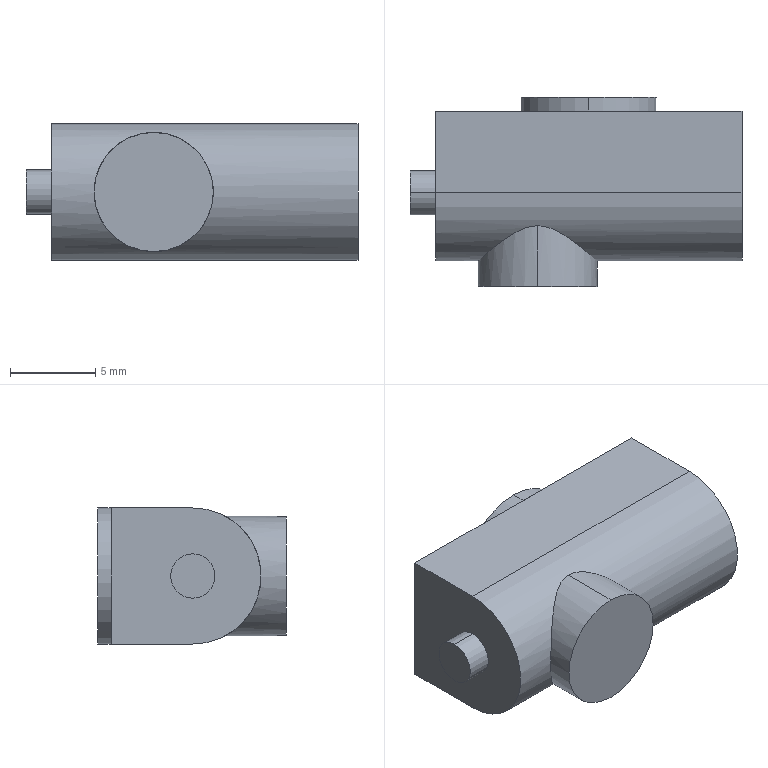Part | STEP file | AFM30-03_AFM3022A Drain_30 | 1 solid | 16 faces | box 19.5 x 11.1 x 8 mm | volume 1266 mm3 | plane 9 | cylinder 7 | commonest cylinder face diameters 8 x3 2.6 x2 7 x2
STEP:
#1=CARTESIAN_POINT('',(-10.5,-5.6,1.3));
#2=VERTEX_POINT('',#1);
#3=CARTESIAN_POINT('',(-10.5,-5.6,-1.3));
#4=VERTEX_POINT('',#3);
#5=CARTESIAN_POINT('',(-10.5,-5.6,0.));
#6=DIRECTION('',(-1.,0.,0.));
#7=DIRECTION('',(0.,0.,1.));
#8=AXIS2_PLACEMENT_3D('',#5,#6,#7);
#9=CIRCLE('',#8,1.3);
#10=EDGE_CURVE('',#2,#4,#9,.T.);
#11=ORIENTED_EDGE('',*,*,#10,.F.);
#12=CARTESIAN_POINT('',(-9.,-5.6,1.3));
#13=VERTEX_POINT('',#12);
#14=CARTESIAN_POINT('',(-10.5,-5.6,1.3));
#15=DIRECTION('',(1.,0.,0.));
#16=VECTOR('',#15,1000.);
#17=LINE('',#14,#16);
#18=EDGE_CURVE('',#2,#13,#17,.T.);
#19=ORIENTED_EDGE('',*,*,#18,.T.);
#20=CARTESIAN_POINT('',(-9.,-5.6,-1.3));
#21=VERTEX_POINT('',#20);
#22=CARTESIAN_POINT('',(-9.,-5.6,0.));
#23=DIRECTION('',(-1.,0.,0.));
#24=DIRECTION('',(0.,0.,-1.));
#25=AXIS2_PLACEMENT_3D('',#22,#23,#24);
#26=CIRCLE('',#25,1.3);
#27=EDGE_CURVE('',#13,#21,#26,.T.);
#28=ORIENTED_EDGE('',*,*,#27,.T.);
#29=CARTESIAN_POINT('',(-10.5,-5.6,-1.3));
#30=DIRECTION('',(1.,0.,0.));
#31=VECTOR('',#30,1000.);
#32=LINE('',#29,#31);
#33=EDGE_CURVE('',#4,#21,#32,.T.);
#34=ORIENTED_EDGE('',*,*,#33,.F.);
#35=EDGE_LOOP('',(#11,#19,#28,#34));
#36=FACE_OUTER_BOUND('',#35,.T.);
#37=CARTESIAN_POINT('',(-10.5,-5.6,0.));
#38=DIRECTION('',(1.,0.,0.));
#39=DIRECTION('',(0.,0.,-1.));
#40=AXIS2_PLACEMENT_3D('',#37,#38,#39);
#41=CYLINDRICAL_SURFACE('',#40,1.3);
#42=ADVANCED_FACE('',(#36),#41,.T.);
#43=CARTESIAN_POINT('',(-3.,-11.1,3.5));
#44=VERTEX_POINT('',#43);
#45=CARTESIAN_POINT('',(-3.,-11.1,-3.5));
#46=VERTEX_POINT('',#45);
#47=CARTESIAN_POINT('',(-3.,-11.1,0.));
#48=DIRECTION('',(0.,1.,0.));
#49=DIRECTION('',(0.,0.,1.));
#50=AXIS2_PLACEMENT_3D('',#47,#48,#49);
#51=CIRCLE('',#50,3.5);
#52=EDGE_CURVE('',#44,#46,#51,.T.);
#53=ORIENTED_EDGE('',*,*,#52,.T.);
#54=CARTESIAN_POINT('',(-3.,-7.536,-3.5));
#55=VERTEX_POINT('',#54);
#56=CARTESIAN_POINT('',(-3.,-11.1,-3.5));
#57=DIRECTION('',(0.,1.,0.));
#58=VECTOR('',#57,1000.);
#59=LINE('',#56,#58);
#60=EDGE_CURVE('',#46,#55,#59,.T.);
#61=ORIENTED_EDGE('',*,*,#60,.T.);
#62=CARTESIAN_POINT('',(-3.,-7.536,3.5));
#63=VERTEX_POINT('',#62);
#64=CARTESIAN_POINT('',(-3.,-7.536,3.5));
#65=CARTESIAN_POINT('',(-2.748,-7.536,3.5));
#66=CARTESIAN_POINT('',(-2.506,-7.587,3.473));
#67=CARTESIAN_POINT('',(-2.044,-7.749,3.375));
#68=CARTESIAN_POINT('',(-1.832,-7.856,3.307));
#69=CARTESIAN_POINT('',(-1.429,-8.088,3.135));
#70=CARTESIAN_POINT('',(-1.239,-8.214,3.032));
#71=CARTESIAN_POINT('',(-0.8859,-8.464,2.797));
#72=CARTESIAN_POINT('',(-0.7207,-8.589,2.665));
#73=CARTESIAN_POINT('',(-0.4108,-8.832,2.365));
#74=CARTESIAN_POINT('',(-0.2662,-8.949,2.197));
#75=CARTESIAN_POINT('',(-0.009917,-9.162,1.833));
#76=CARTESIAN_POINT('',(0.1038,-9.258,1.635));
#77=CARTESIAN_POINT('',(0.295,-9.422,1.203));
#78=CARTESIAN_POINT('',(0.3697,-9.486,0.9771));
#79=CARTESIAN_POINT('',(0.4469,-9.554,0.6193));
#80=CARTESIAN_POINT('',(0.4669,-9.571,0.4961));
#81=CARTESIAN_POINT('',(0.4932,-9.594,0.2506));
#82=CARTESIAN_POINT('',(0.4998,-9.6,0.1277));
#83=CARTESIAN_POINT('',(0.5003,-9.6,-0.2418));
#84=CARTESIAN_POINT('',(0.4737,-9.577,-0.4926));
#85=CARTESIAN_POINT('',(0.372,-9.488,-0.9689));
#86=CARTESIAN_POINT('',(0.2966,-9.423,-1.199));
#87=CARTESIAN_POINT('',(0.01172,-9.179,-1.844));
#88=CARTESIAN_POINT('',(-0.2543,-8.954,-2.213));
#89=CARTESIAN_POINT('',(-0.7164,-8.593,-2.661));
#90=CARTESIAN_POINT('',(-0.882,-8.467,-2.795));
#91=CARTESIAN_POINT('',(-1.24,-8.214,-3.033));
#92=CARTESIAN_POINT('',(-1.428,-8.089,-3.134));
#93=CARTESIAN_POINT('',(-1.829,-7.857,-3.305));
#94=CARTESIAN_POINT('',(-2.045,-7.749,-3.375));
#95=CARTESIAN_POINT('',(-2.39,-7.628,-3.448));
#96=CARTESIAN_POINT('',(-2.508,-7.594,-3.467));
#97=CARTESIAN_POINT('',(-2.752,-7.549,-3.493));
#98=CARTESIAN_POINT('',(-2.877,-7.536,-3.5));
#99=CARTESIAN_POINT('',(-3.,-7.536,-3.5));
#100=B_SPLINE_CURVE_WITH_KNOTS('',3,(#64,#65,#66,#67,#68,#69,#70,#71,#72,#73,#74,#75,#76,#77,#78,#79,#80,#81,#82,#83,#84,#85,#86,#87,#88,#89,#90,#91,#92,#93,#94,#95,#96,#97,#98,#99),.UNSPECIFIED.,.F.,.F.,(4,2,2,2,2,2,2,2,2,2,2,2,2,2,2,2,2,4),(0.,0.0007411,0.001482,0.002223,0.002964,0.003705,0.004446,0.005188,0.005558,0.005929,0.00667,0.007411,0.008893,0.009634,0.01038,0.01112,0.01149,0.01186),.UNSPECIFIED.);
#101=EDGE_CURVE('',#63,#55,#100,.T.);
#102=ORIENTED_EDGE('',*,*,#101,.F.);
#103=CARTESIAN_POINT('',(-3.,-11.1,3.5));
#104=DIRECTION('',(0.,1.,0.));
#105=VECTOR('',#104,1000.);
#106=LINE('',#103,#105);
#107=EDGE_CURVE('',#44,#63,#106,.T.);
#108=ORIENTED_EDGE('',*,*,#107,.F.);
#109=EDGE_LOOP('',(#53,#61,#102,#108));
#110=FACE_OUTER_BOUND('',#109,.T.);
#111=CARTESIAN_POINT('',(-3.,-11.1,0.));
#112=DIRECTION('',(0.,1.,0.));
#113=DIRECTION('',(0.,0.,1.));
#114=AXIS2_PLACEMENT_3D('',#111,#112,#113);
#115=CYLINDRICAL_SURFACE('',#114,3.5);
#116=ADVANCED_FACE('',(#110),#115,.T.);
#117=CARTESIAN_POINT('',(0.,-0.8,4.));
#118=VERTEX_POINT('',#117);
#119=CARTESIAN_POINT('',(0.,-0.8,-4.));
#120=VERTEX_POINT('',#119);
#121=CARTESIAN_POINT('',(0.,-0.8,0.));
#122=DIRECTION('',(0.,1.,0.));
#123=DIRECTION('',(0.,0.,1.));
#124=AXIS2_PLACEMENT_3D('',#121,#122,#123);
#125=CIRCLE('',#124,4.);
#126=EDGE_CURVE('',#118,#120,#125,.T.);
#127=ORIENTED_EDGE('',*,*,#126,.T.);
#128=CARTESIAN_POINT('',(0.,0.,-4.));
#129=VERTEX_POINT('',#128);
#130=CARTESIAN_POINT('',(0.,-0.8,-4.));
#131=DIRECTION('',(0.,1.,0.));
#132=VECTOR('',#131,1000.);
#133=LINE('',#130,#132);
#134=EDGE_CURVE('',#120,#129,#133,.T.);
#135=ORIENTED_EDGE('',*,*,#134,.T.);
#136=CARTESIAN_POINT('',(0.,0.,4.));
#137=VERTEX_POINT('',#136);
#138=CARTESIAN_POINT('',(0.,0.,0.));
#139=DIRECTION('',(0.,1.,0.));
#140=DIRECTION('',(0.,0.,1.));
#141=AXIS2_PLACEMENT_3D('',#138,#139,#140);
#142=CIRCLE('',#141,4.);
#143=EDGE_CURVE('',#137,#129,#142,.T.);
#144=ORIENTED_EDGE('',*,*,#143,.F.);
#145=CARTESIAN_POINT('',(0.,-0.8,4.));
#146=DIRECTION('',(0.,1.,0.));
#147=VECTOR('',#146,1000.);
#148=LINE('',#145,#147);
#149=EDGE_CURVE('',#118,#137,#148,.T.);
#150=ORIENTED_EDGE('',*,*,#149,.F.);
#151=EDGE_LOOP('',(#127,#135,#144,#150));
#152=FACE_OUTER_BOUND('',#151,.T.);
#153=CARTESIAN_POINT('',(0.,-0.8,0.));
#154=DIRECTION('',(0.,1.,0.));
#155=DIRECTION('',(0.,0.,1.));
#156=AXIS2_PLACEMENT_3D('',#153,#154,#155);
#157=CYLINDRICAL_SURFACE('',#156,4.);
#158=ADVANCED_FACE('',(#152),#157,.T.);
#159=CARTESIAN_POINT('',(-9.,-0.8,-4.));
#160=VERTEX_POINT('',#159);
#161=CARTESIAN_POINT('',(-9.,-0.8,4.));
#162=VERTEX_POINT('',#161);
#163=CARTESIAN_POINT('',(-9.,-0.8,4.));
#164=DIRECTION('',(0.,0.,1.));
#165=VECTOR('',#164,1000.);
#166=LINE('',#163,#165);
#167=EDGE_CURVE('',#160,#162,#166,.T.);
#168=ORIENTED_EDGE('',*,*,#167,.F.);
#169=CARTESIAN_POINT('',(-9.,-5.6,-4.));
#170=VERTEX_POINT('',#169);
#171=CARTESIAN_POINT('',(-9.,-0.8,-4.));
#172=DIRECTION('',(0.,1.,0.));
#173=VECTOR('',#172,1000.);
#174=LINE('',#171,#173);
#175=EDGE_CURVE('',#170,#160,#174,.T.);
#176=ORIENTED_EDGE('',*,*,#175,.F.);
#177=CARTESIAN_POINT('',(-9.,-5.6,4.));
#178=VERTEX_POINT('',#177);
#179=CARTESIAN_POINT('',(-9.,-5.6,0.));
#180=DIRECTION('',(1.,0.,0.));
#181=DIRECTION('',(0.,0.,-1.));
#182=AXIS2_PLACEMENT_3D('',#179,#180,#181);
#183=CIRCLE('',#182,4.);
#184=EDGE_CURVE('',#178,#170,#183,.T.);
#185=ORIENTED_EDGE('',*,*,#184,.F.);
#186=CARTESIAN_POINT('',(-9.,-0.8,4.));
#187=DIRECTION('',(0.,-1.,0.));
#188=VECTOR('',#187,1000.);
#189=LINE('',#186,#188);
#190=EDGE_CURVE('',#162,#178,#189,.T.);
#191=ORIENTED_EDGE('',*,*,#190,.F.);
#192=EDGE_LOOP('',(#168,#176,#185,#191));
#193=FACE_OUTER_BOUND('',#192,.T.);
#194=CARTESIAN_POINT('',(-9.,-5.6,0.));
#195=DIRECTION('',(-1.,0.,0.));
#196=DIRECTION('',(0.,0.,-1.));
#197=AXIS2_PLACEMENT_3D('',#194,#195,#196);
#198=CIRCLE('',#197,1.3);
#199=EDGE_CURVE('',#21,#13,#198,.T.);
#200=ORIENTED_EDGE('',*,*,#199,.F.);
#201=ORIENTED_EDGE('',*,*,#27,.F.);
#202=EDGE_LOOP('',(#200,#201));
#203=FACE_BOUND('',#202,.T.);
#204=CARTESIAN_POINT('',(-9.,-5.6,0.));
#205=DIRECTION('',(1.,0.,0.));
#206=DIRECTION('',(0.,0.,-1.));
#207=AXIS2_PLACEMENT_3D('',#204,#205,#206);
#208=PLANE('',#207);
#209=ADVANCED_FACE('',(#193,#203),#208,.F.);
#210=ORIENTED_EDGE('',*,*,#134,.F.);
#211=CARTESIAN_POINT('',(0.,-0.8,0.));
#212=DIRECTION('',(0.,1.,0.));
#213=DIRECTION('',(0.,0.,1.));
#214=AXIS2_PLACEMENT_3D('',#211,#212,#213);
#215=CIRCLE('',#214,4.);
#216=EDGE_CURVE('',#120,#118,#215,.T.);
#217=ORIENTED_EDGE('',*,*,#216,.T.);
#218=ORIENTED_EDGE('',*,*,#149,.T.);
#219=CARTESIAN_POINT('',(0.,0.,0.));
#220=DIRECTION('',(0.,1.,0.));
#221=DIRECTION('',(0.,0.,1.));
#222=AXIS2_PLACEMENT_3D('',#219,#220,#221);
#223=CIRCLE('',#222,4.);
#224=EDGE_CURVE('',#129,#137,#223,.T.);
#225=ORIENTED_EDGE('',*,*,#224,.F.);
#226=EDGE_LOOP('',(#210,#217,#218,#225));
#227=FACE_OUTER_BOUND('',#226,.T.);
#228=CARTESIAN_POINT('',(0.,-0.8,0.));
#229=DIRECTION('',(0.,1.,0.));
#230=DIRECTION('',(0.,0.,1.));
#231=AXIS2_PLACEMENT_3D('',#228,#229,#230);
#232=CYLINDRICAL_SURFACE('',#231,4.);
#233=ADVANCED_FACE('',(#227),#232,.T.);
#234=ORIENTED_EDGE('',*,*,#143,.T.);
#235=ORIENTED_EDGE('',*,*,#224,.T.);
#236=EDGE_LOOP('',(#234,#235));
#237=FACE_OUTER_BOUND('',#236,.T.);
#238=CARTESIAN_POINT('',(0.,0.,0.));
#239=DIRECTION('',(0.,1.,0.));
#240=DIRECTION('',(0.,0.,1.));
#241=AXIS2_PLACEMENT_3D('',#238,#239,#240);
#242=PLANE('',#241);
#243=ADVANCED_FACE('',(#237),#242,.T.);
#244=ORIENTED_EDGE('',*,*,#126,.F.);
#245=CARTESIAN_POINT('',(9.,-0.8,4.));
#246=VERTEX_POINT('',#245);
#247=CARTESIAN_POINT('',(9.,-0.8,4.));
#248=DIRECTION('',(-1.,0.,0.));
#249=VECTOR('',#248,1000.);
#250=LINE('',#247,#249);
#251=EDGE_CURVE('',#246,#118,#250,.T.);
#252=ORIENTED_EDGE('',*,*,#251,.F.);
#253=CARTESIAN_POINT('',(9.,-0.8,-4.));
#254=VERTEX_POINT('',#253);
#255=CARTESIAN_POINT('',(9.,-0.8,4.));
#256=DIRECTION('',(0.,0.,1.));
#257=VECTOR('',#256,1000.);
#258=LINE('',#255,#257);
#259=EDGE_CURVE('',#254,#246,#258,.T.);
#260=ORIENTED_EDGE('',*,*,#259,.F.);
#261=CARTESIAN_POINT('',(9.,-0.8,-4.));
#262=DIRECTION('',(-1.,0.,0.));
#263=VECTOR('',#262,1000.);
#264=LINE('',#261,#263);
#265=EDGE_CURVE('',#254,#120,#264,.T.);
#266=ORIENTED_EDGE('',*,*,#265,.T.);
#267=EDGE_LOOP('',(#244,#252,#260,#266));
#268=FACE_OUTER_BOUND('',#267,.T.);
#269=CARTESIAN_POINT('',(9.,-0.8,4.));
#270=DIRECTION('',(0.,-1.,0.));
#271=DIRECTION('',(0.,0.,-1.));
#272=AXIS2_PLACEMENT_3D('',#269,#270,#271);
#273=PLANE('',#272);
#274=ADVANCED_FACE('',(#268),#273,.F.);
#275=CARTESIAN_POINT('',(9.,-0.8,4.));
#276=DIRECTION('',(-1.,0.,0.));
#277=VECTOR('',#276,1000.);
#278=LINE('',#275,#277);
#279=EDGE_CURVE('',#118,#162,#278,.T.);
#280=ORIENTED_EDGE('',*,*,#279,.F.);
#281=ORIENTED_EDGE('',*,*,#216,.F.);
#282=CARTESIAN_POINT('',(9.,-0.8,-4.));
#283=DIRECTION('',(-1.,0.,0.));
#284=VECTOR('',#283,1000.);
#285=LINE('',#282,#284);
#286=EDGE_CURVE('',#120,#160,#285,.T.);
#287=ORIENTED_EDGE('',*,*,#286,.T.);
#288=ORIENTED_EDGE('',*,*,#167,.T.);
#289=EDGE_LOOP('',(#280,#281,#287,#288));
#290=FACE_OUTER_BOUND('',#289,.T.);
#291=CARTESIAN_POINT('',(9.,-0.8,4.));
#292=DIRECTION('',(0.,-1.,0.));
#293=DIRECTION('',(0.,0.,-1.));
#294=AXIS2_PLACEMENT_3D('',#291,#292,#293);
#295=PLANE('',#294);
#296=ADVANCED_FACE('',(#290),#295,.F.);
#297=ORIENTED_EDGE('',*,*,#190,.T.);
#298=CARTESIAN_POINT('',(9.,-5.6,4.));
#299=VERTEX_POINT('',#298);
#300=CARTESIAN_POINT('',(9.,-5.6,4.));
#301=DIRECTION('',(-1.,0.,0.));
#302=VECTOR('',#301,1000.);
#303=LINE('',#300,#302);
#304=EDGE_CURVE('',#299,#178,#303,.T.);
#305=ORIENTED_EDGE('',*,*,#304,.F.);
#306=CARTESIAN_POINT('',(9.,-0.8,4.));
#307=DIRECTION('',(0.,-1.,0.));
#308=VECTOR('',#307,1000.);
#309=LINE('',#306,#308);
#310=EDGE_CURVE('',#246,#299,#309,.T.);
#311=ORIENTED_EDGE('',*,*,#310,.F.);
#312=ORIENTED_EDGE('',*,*,#251,.T.);
#313=ORIENTED_EDGE('',*,*,#279,.T.);
#314=EDGE_LOOP('',(#297,#305,#311,#312,#313));
#315=FACE_OUTER_BOUND('',#314,.T.);
#316=CARTESIAN_POINT('',(9.,-0.8,4.));
#317=DIRECTION('',(0.,0.,-1.));
#318=DIRECTION('',(0.,1.,0.));
#319=AXIS2_PLACEMENT_3D('',#316,#317,#318);
#320=PLANE('',#319);
#321=ADVANCED_FACE('',(#315),#320,.F.);
#322=ORIENTED_EDGE('',*,*,#101,.T.);
#323=CARTESIAN_POINT('',(-3.,-7.536,-3.5));
#324=CARTESIAN_POINT('',(-3.247,-7.536,-3.5));
#325=CARTESIAN_POINT('',(-3.495,-7.587,-3.473));
#326=CARTESIAN_POINT('',(-3.953,-7.748,-3.376));
#327=CARTESIAN_POINT('',(-4.17,-7.857,-3.306));
#328=CARTESIAN_POINT('',(-4.571,-8.089,-3.135));
#329=CARTESIAN_POINT('',(-4.759,-8.213,-3.034));
#330=CARTESIAN_POINT('',(-5.115,-8.464,-2.797));
#331=CARTESIAN_POINT('',(-5.282,-8.592,-2.662));
#332=CARTESIAN_POINT('',(-5.59,-8.833,-2.363));
#333=CARTESIAN_POINT('',(-5.732,-8.948,-2.199));
#334=CARTESIAN_POINT('',(-5.99,-9.162,-1.832));
#335=CARTESIAN_POINT('',(-6.105,-9.259,-1.632));
#336=CARTESIAN_POINT('',(-6.294,-9.421,-1.206));
#337=CARTESIAN_POINT('',(-6.37,-9.487,-0.9741));
#338=CARTESIAN_POINT('',(-6.473,-9.576,-0.4995));
#339=CARTESIAN_POINT('',(-6.5,-9.6,-0.2562));
#340=CARTESIAN_POINT('',(-6.5,-9.6,0.2437));
#341=CARTESIAN_POINT('',(-6.474,-9.577,0.4897));
#342=CARTESIAN_POINT('',(-6.373,-9.489,0.967));
#343=CARTESIAN_POINT('',(-6.297,-9.423,1.198));
#344=CARTESIAN_POINT('',(-6.108,-9.261,1.627));
#345=CARTESIAN_POINT('',(-5.993,-9.164,1.829));
#346=CARTESIAN_POINT('',(-5.736,-8.951,2.194));
#347=CARTESIAN_POINT('',(-5.594,-8.836,2.359));
#348=CARTESIAN_POINT('',(-5.285,-8.593,2.66));
#349=CARTESIAN_POINT('',(-5.117,-8.466,2.796));
#350=CARTESIAN_POINT('',(-4.762,-8.215,3.031));
#351=CARTESIAN_POINT('',(-4.575,-8.091,3.133));
#352=CARTESIAN_POINT('',(-4.171,-7.857,3.306));
#353=CARTESIAN_POINT('',(-3.956,-7.749,3.375));
#354=CARTESIAN_POINT('',(-3.611,-7.628,3.448));
#355=CARTESIAN_POINT('',(-3.491,-7.594,3.468));
#356=CARTESIAN_POINT('',(-3.249,-7.549,3.493));
#357=CARTESIAN_POINT('',(-3.126,-7.536,3.5));
#358=CARTESIAN_POINT('',(-3.,-7.536,3.5));
#359=B_SPLINE_CURVE_WITH_KNOTS('',3,(#323,#324,#325,#326,#327,#328,#329,#330,#331,#332,#333,#334,#335,#336,#337,#338,#339,#340,#341,#342,#343,#344,#345,#346,#347,#348,#349,#350,#351,#352,#353,#354,#355,#356,#357,#358),.UNSPECIFIED.,.F.,.F.,(4,2,2,2,2,2,2,2,2,2,2,2,2,2,2,2,2,4),(0.01186,0.0126,0.01334,0.01408,0.01482,0.01556,0.0163,0.01704,0.01778,0.01853,0.01927,0.02001,0.02075,0.02149,0.02223,0.02297,0.02334,0.02371),.UNSPECIFIED.);
#360=EDGE_CURVE('',#55,#63,#359,.T.);
#361=ORIENTED_EDGE('',*,*,#360,.T.);
#362=EDGE_LOOP('',(#322,#361));
#363=FACE_BOUND('',#362,.T.);
#364=ORIENTED_EDGE('',*,*,#184,.T.);
#365=CARTESIAN_POINT('',(9.,-5.6,-4.));
#366=VERTEX_POINT('',#365);
#367=CARTESIAN_POINT('',(9.,-5.6,-4.));
#368=DIRECTION('',(-1.,0.,0.));
#369=VECTOR('',#368,1000.);
#370=LINE('',#367,#369);
#371=EDGE_CURVE('',#366,#170,#370,.T.);
#372=ORIENTED_EDGE('',*,*,#371,.F.);
#373=CARTESIAN_POINT('',(9.,-5.6,0.));
#374=DIRECTION('',(1.,0.,0.));
#375=DIRECTION('',(0.,0.,-1.));
#376=AXIS2_PLACEMENT_3D('',#373,#374,#375);
#377=CIRCLE('',#376,4.);
#378=EDGE_CURVE('',#299,#366,#377,.T.);
#379=ORIENTED_EDGE('',*,*,#378,.F.);
#380=ORIENTED_EDGE('',*,*,#304,.T.);
#381=EDGE_LOOP('',(#364,#372,#379,#380));
#382=FACE_OUTER_BOUND('',#381,.T.);
#383=CARTESIAN_POINT('',(9.,-5.6,0.));
#384=DIRECTION('',(-1.,0.,0.));
#385=DIRECTION('',(0.,0.,1.));
#386=AXIS2_PLACEMENT_3D('',#383,#384,#385);
#387=CYLINDRICAL_SURFACE('',#386,4.);
#388=ADVANCED_FACE('',(#363,#382),#387,.T.);
#389=ORIENTED_EDGE('',*,*,#175,.T.);
#390=ORIENTED_EDGE('',*,*,#286,.F.);
#391=ORIENTED_EDGE('',*,*,#265,.F.);
#392=CARTESIAN_POINT('',(9.,-0.8,-4.));
#393=DIRECTION('',(0.,1.,0.));
#394=VECTOR('',#393,1000.);
#395=LINE('',#392,#394);
#396=EDGE_CURVE('',#366,#254,#395,.T.);
#397=ORIENTED_EDGE('',*,*,#396,.F.);
#398=ORIENTED_EDGE('',*,*,#371,.T.);
#399=EDGE_LOOP('',(#389,#390,#391,#397,#398));
#400=FACE_OUTER_BOUND('',#399,.T.);
#401=CARTESIAN_POINT('',(9.,-0.8,-4.));
#402=DIRECTION('',(0.,0.,1.));
#403=DIRECTION('',(0.,-1.,0.));
#404=AXIS2_PLACEMENT_3D('',#401,#402,#403);
#405=PLANE('',#404);
#406=ADVANCED_FACE('',(#400),#405,.F.);
#407=ORIENTED_EDGE('',*,*,#259,.T.);
#408=ORIENTED_EDGE('',*,*,#310,.T.);
#409=ORIENTED_EDGE('',*,*,#378,.T.);
#410=ORIENTED_EDGE('',*,*,#396,.T.);
#411=EDGE_LOOP('',(#407,#408,#409,#410));
#412=FACE_OUTER_BOUND('',#411,.T.);
#413=CARTESIAN_POINT('',(9.,-5.6,0.));
#414=DIRECTION('',(1.,0.,0.));
#415=DIRECTION('',(0.,0.,-1.));
#416=AXIS2_PLACEMENT_3D('',#413,#414,#415);
#417=PLANE('',#416);
#418=ADVANCED_FACE('',(#412),#417,.T.);
#419=ORIENTED_EDGE('',*,*,#60,.F.);
#420=CARTESIAN_POINT('',(-3.,-11.1,0.));
#421=DIRECTION('',(0.,1.,0.));
#422=DIRECTION('',(0.,0.,1.));
#423=AXIS2_PLACEMENT_3D('',#420,#421,#422);
#424=CIRCLE('',#423,3.5);
#425=EDGE_CURVE('',#46,#44,#424,.T.);
#426=ORIENTED_EDGE('',*,*,#425,.T.);
#427=ORIENTED_EDGE('',*,*,#107,.T.);
#428=ORIENTED_EDGE('',*,*,#360,.F.);
#429=EDGE_LOOP('',(#419,#426,#427,#428));
#430=FACE_OUTER_BOUND('',#429,.T.);
#431=CARTESIAN_POINT('',(-3.,-11.1,0.));
#432=DIRECTION('',(0.,1.,0.));
#433=DIRECTION('',(0.,0.,1.));
#434=AXIS2_PLACEMENT_3D('',#431,#432,#433);
#435=CYLINDRICAL_SURFACE('',#434,3.5);
#436=ADVANCED_FACE('',(#430),#435,.T.);
#437=ORIENTED_EDGE('',*,*,#52,.F.);
#438=ORIENTED_EDGE('',*,*,#425,.F.);
#439=EDGE_LOOP('',(#437,#438));
#440=FACE_OUTER_BOUND('',#439,.T.);
#441=CARTESIAN_POINT('',(-3.,-11.1,0.));
#442=DIRECTION('',(0.,1.,0.));
#443=DIRECTION('',(0.,0.,1.));
#444=AXIS2_PLACEMENT_3D('',#441,#442,#443);
#445=PLANE('',#444);
#446=ADVANCED_FACE('',(#440),#445,.F.);
#447=ORIENTED_EDGE('',*,*,#18,.F.);
#448=CARTESIAN_POINT('',(-10.5,-5.6,0.));
#449=DIRECTION('',(-1.,0.,0.));
#450=DIRECTION('',(0.,0.,1.));
#451=AXIS2_PLACEMENT_3D('',#448,#449,#450);
#452=CIRCLE('',#451,1.3);
#453=EDGE_CURVE('',#4,#2,#452,.T.);
#454=ORIENTED_EDGE('',*,*,#453,.F.);
#455=ORIENTED_EDGE('',*,*,#33,.T.);
#456=ORIENTED_EDGE('',*,*,#199,.T.);
#457=EDGE_LOOP('',(#447,#454,#455,#456));
#458=FACE_OUTER_BOUND('',#457,.T.);
#459=CARTESIAN_POINT('',(-10.5,-5.6,0.));
#460=DIRECTION('',(1.,0.,0.));
#461=DIRECTION('',(0.,0.,-1.));
#462=AXIS2_PLACEMENT_3D('',#459,#460,#461);
#463=CYLINDRICAL_SURFACE('',#462,1.3);
#464=ADVANCED_FACE('',(#458),#463,.T.);
#465=ORIENTED_EDGE('',*,*,#453,.T.);
#466=ORIENTED_EDGE('',*,*,#10,.T.);
#467=EDGE_LOOP('',(#465,#466));
#468=FACE_OUTER_BOUND('',#467,.T.);
#469=CARTESIAN_POINT('',(-10.5,-5.6,0.));
#470=DIRECTION('',(-1.,0.,0.));
#471=DIRECTION('',(0.,0.,1.));
#472=AXIS2_PLACEMENT_3D('',#469,#470,#471);
#473=PLANE('',#472);
#474=ADVANCED_FACE('',(#468),#473,.T.);
#475=CLOSED_SHELL('',(#42,#116,#158,#209,#233,#243,#274,#296,#321,#388,#406,#418,#436,#446,#464,#474));
#476=MANIFOLD_SOLID_BREP('',#475);
#477=CARTESIAN_POINT('',(0.,0.,0.));
#478=DIRECTION('',(0.,0.,1.));
#479=DIRECTION('',(1.,0.,0.));
#480=AXIS2_PLACEMENT_3D('',#477,#478,#479);
#481=(LENGTH_UNIT()NAMED_UNIT(*)SI_UNIT(.MILLI.,.METRE.));
#482=UNCERTAINTY_MEASURE_WITH_UNIT(LENGTH_MEASURE(0.00001),#481,'','');
#483=(NAMED_UNIT(*)PLANE_ANGLE_UNIT()SI_UNIT($,.RADIAN.));
#484=(NAMED_UNIT(*)SI_UNIT($,.STERADIAN.)SOLID_ANGLE_UNIT());
#485=(GEOMETRIC_REPRESENTATION_CONTEXT(3)GLOBAL_UNCERTAINTY_ASSIGNED_CONTEXT((#482))GLOBAL_UNIT_ASSIGNED_CONTEXT((#481,#483,#484))REPRESENTATION_CONTEXT('',''));
#486=ADVANCED_BREP_SHAPE_REPRESENTATION('',(#476,#480),#485);